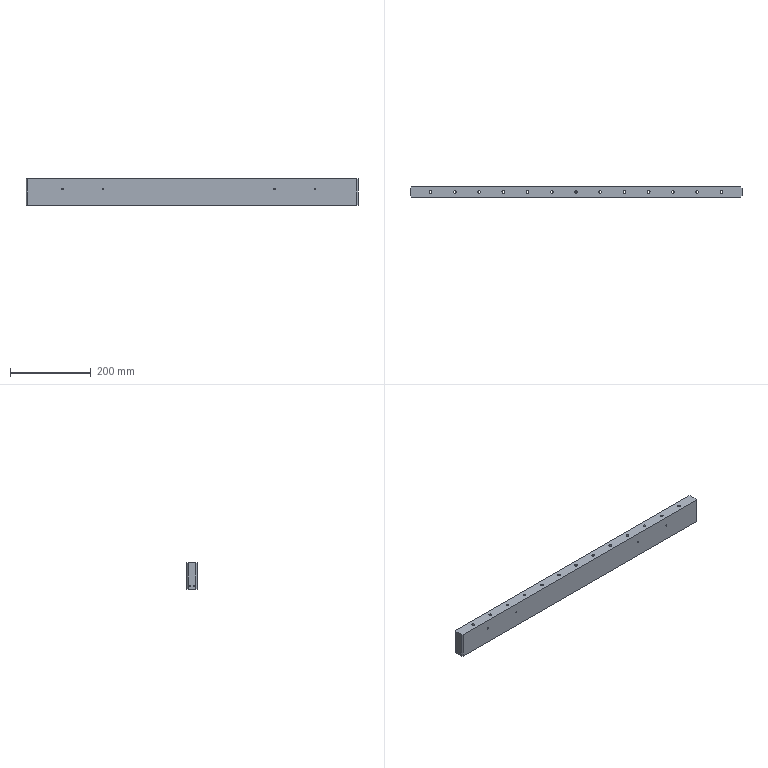Part | NX | 1 solid | 89 faces | box 822 x 25 x 65 mm | volume 1270022 mm3 | cylinder 48 | plane 23 | cone 18 | commonest cylinder face diameters 4.2 x14 6.6 x13 11 x13 3.3 x8